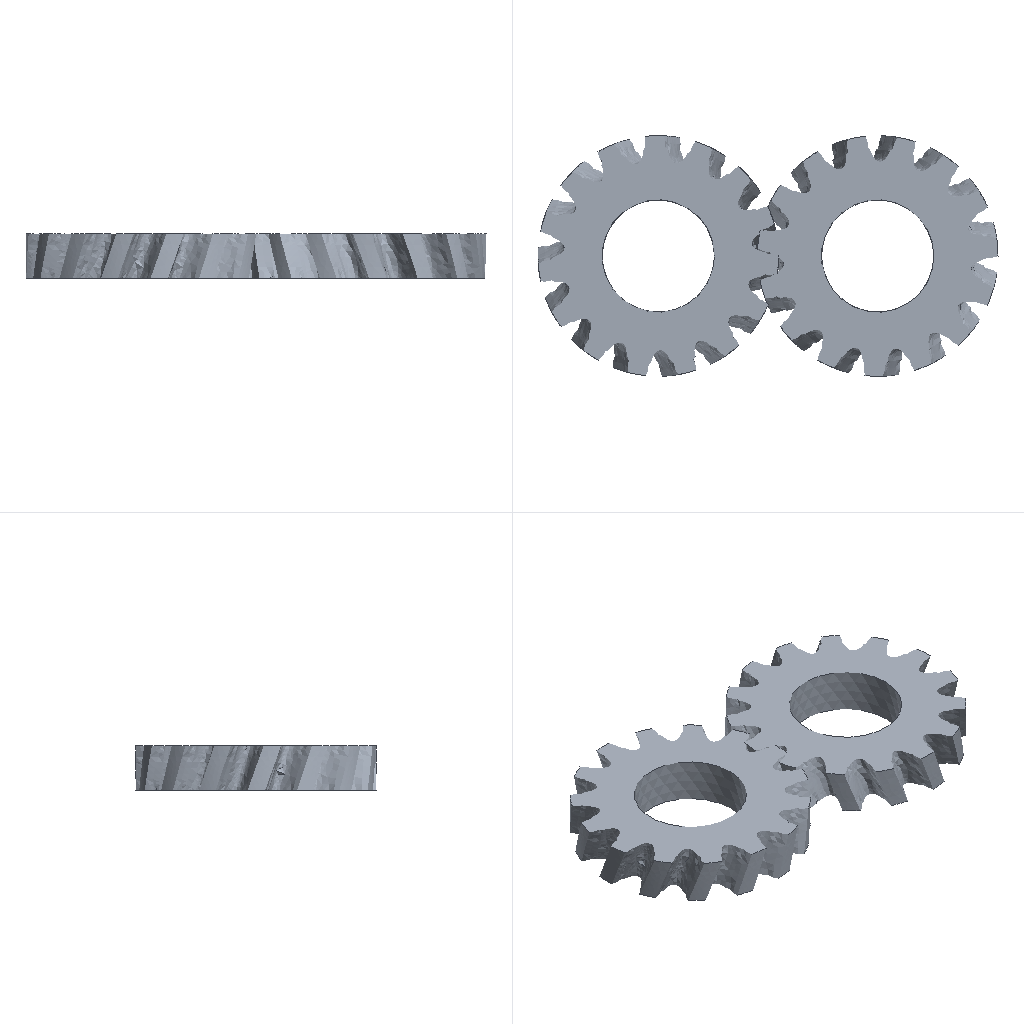Simulation study | ansys workbench
Ansys APDL input file, long lists of numbers shortened:
/batch
/config,noeldb,1     ! force off writing results to database
*get,_wallstrt,active,,time,wall
! ANSYS input file written by Workbench version 16.0 RELEASE
! File used for geometry attach: C:\Users\hmm\AppData\Local\Temp\WB_LAPTOP-92PEKBNI_hmm_19940_2\unsaved_project_files\dp0\SYS\DM\SYS.agdb
/title,unsaved_project--Static Structural (A5)
*DIM,_wb_ProjectScratch_dir,string,248
_wb_ProjectScratch_dir(1) = 'C:\Users\hmm\AppData\Local\Temp\WB_LAPTOP-92PEKBNI_hmm_19940_2\_ProjectScratch\Scr7DD3\'
*DIM,_wb_SolverFiles_dir,string,248
_wb_SolverFiles_dir(1) = 'C:\Users\hmm\AppData\Local\Temp\WB_LAPTOP-92PEKBNI_hmm_19940_2\unsaved_project_files\dp0\SYS\MECH\'
*DIM,_wb_userfiles_dir,string,248
_wb_userfiles_dir(1) = 'C:\Users\hmm\AppData\Local\Temp\WB_LAPTOP-92PEKBNI_hmm_19940_2\unsaved_project_files\user_files\'
/com,--- Data in consistent NMM units. See Solving Units in the help system for more information.
/units,MPA
/nopr
/wb,file,start              !  signify a WB generated input file
/prep7
! Turn off shape checking because checks already performed inside WB mesher.
! See help system for more information.
SHPP,OFF,,NOWARN
/nolist
etcon,set             ! allow ANSYS to choose best KEYOP's for 180x elements
/com,*********** Nodes for the whole assembly ***********
nblock,3
(1i9,3e20.9e3)
        1    6.183845739E+001   -1.519273240E+001    4.233906430E+000
! (51987 more lines like these left out)
-1
/wb,elem,start            !  set before creation of elements
/com,*********** Elements for Body 1 "Solid" ***********
et,1,187
eblock,19,solid,,11470
(19i9)
        1        1        1        1        0        0        0        0       10        0        1        2        8      444        9     4085     4078     4145     4116
! (22939 more lines like these left out)
-1
/com,*********** Elements for Body 2 "Solid" ***********
et,2,187
eblock,19,solid,,14800
(19i9)
        2        2        2        2        0        0        0        0       10        0    11471    23126    24680    25907    25826    28074    45158    28065    28080
! (29599 more lines like these left out)
-1
/wb,elem,end               !  done creating elements
/com,*********** Send User Defined Coordinate System(s) ***********
local,12,0,48.804,3.57140444047492e-015,5.,-0.,0.,0.
local,13,0,0.,-7.65404249467096e-016,5.,-0.,0.,0.
csys,0
toffst,273.15,  ! Temperature offset from absolute zero
/com,*********** Set Reference Temperature ***********
tref,22.
/wb,mat,start              !  starting to send materials
/com,*********** Send Materials ***********
MP,DENS,1,7.85e-09,	! tonne mm^-3
MP,ALPX,1,1.2e-05,	! C^-1
MP,C,1,434000000,	! mm^2 s^-2 C^-1
MP,KXX,1,60.5,	! tonne mm s^-3 C^-1
MP,RSVX,1,0.00017,	! ohm mm
MP,EX,1,200000,	! tonne s^-2 mm^-1
MP,NUXY,1,0.3,
MP,MURX,1,10000,
MP,DENS,2,7.85e-09,	! tonne mm^-3
MP,ALPX,2,1.2e-05,	! C^-1
MP,C,2,434000000,	! mm^2 s^-2 C^-1
MP,KXX,2,60.5,	! tonne mm s^-3 C^-1
MP,RSVX,2,0.00017,	! ohm mm
MP,EX,2,200000,	! tonne s^-2 mm^-1
MP,NUXY,2,0.3,
MP,MURX,2,10000,
/wb,mat,end                !  done sending materials
!************************* Model Summary ********************
!Solid,	Structural Steel,	matid,	1
!Solid,	Structural Steel,	matid,	2
!************************* End Model Summary ********************
! get the diagonal of the bounding box. Needed later for other things
*get,_xmin,node,,mnloc,x
*get,_ymin,node,,mnloc,y
*get,_zmin,node,,mnloc,z
*get,_xmax,node,,mxloc,x
*get,_ymax,node,,mxloc,y
*get,_zmax,node,,mxloc,z
_ASMDIAG=(_xmax-_xmin)*(_xmax-_xmin)+(_ymax-_ymin)*(_ymax-_ymin)+(_zmax-_zmin)*(_zmax-_zmin)
_ASMDIAG=SQRT(_ASMDIAG)
/wb,contact,start          !  starting to send contact
/com,*********** Create Contact "Frictional - No Selection To No Selection" ***********
/com,            Real Constant Set For Above Contact Is 4 & 3
*set,tid,4
*set,cid,3
r,tid
r,cid
et,tid,170
et,cid,174
eblock,10,,,3036
(15i9)
    26277        4        4        4        0     2495     2490     2493     2493    16197    16195     2493    16196
! (3035 more lines like these left out)
-1
eblock,10,,,3036
(15i9)
    29313        3        3        3        0     2495     2490     2493     2493    16197    16195     2493    16196
! (3035 more lines like these left out)
-1
eblock,10,,,4294
(15i9)
    32349        3        4        3        0    26571    26575    26578    26578    44256    44254    26578    44255
! (4293 more lines like these left out)
-1
eblock,10,,,4294
(15i9)
    36643        4        3        4        0    26571    26575    26578    26578    44256    44254    26578    44255
! (4293 more lines like these left out)
-1
keyo,cid,8,2               ! auto create asymmetric contact (from Program Controlled setting)
keyo,cid,10,2              ! adjust contact stiffness each NR iteration (from Program Controlled setting)
keyo,cid,12,0              ! standard contact
mp,mu,cid,0.1	! unitless
keyo,cid,2,0               ! augmented Lagrange (from Program Controlled setting)
keyo,cid,4,0               ! on Gauss point (from Program Controlled setting)
keyo,cid,9,0               ! use real geometry with stepped effects
keyo,cid,7,0               ! No Prediction
rmod,tid,3,1.	! FKN
rmod,tid,5,0.	! ICONT
rmod,tid,6,0.	! PINB
rmod,tid,10,0.	! CNOF
rmod,tid,12,0.	! FKT
rmod,tid,36,44	! WB DSID
rmod,cid,3,1.	! FKN
rmod,cid,5,0.	! ICONT
rmod,cid,6,0.	! PINB
rmod,cid,10,0.	! CNOF
rmod,cid,12,0.	! FKT
rmod,cid,36,44	! WB DSID
nsel,all
esel,all
/wb,contact,end            !  done creating contacts
/com,*********** Send Named Selection as Node Component ***********
CMBLOCK,SELECTION,NODE,     6867
(8i10)
        11        12       433       434       435       436       437       438
! (858 more lines like these left out)
/com,*********** Send Named Selection as Node Component ***********
CMBLOCK,SELECTION_2,NODE,     9383
(8i10)
     23134     23135     23141     23142     23143     23158     23169     23195
! (1172 more lines like these left out)
/golist
/wb,load,start             !  starting to send loads
nsel,all
/com,*********** Create Remote Point "Internal Remote Point 2" ***********
! -------- Remote Point Used by "Revolute - Ground To Solid" --------
*set,tid,6
*set,cid,5
et,cid,174
et,tid,170
keyo,tid,2,1               ! Don't fix the pilot node
keyo,tid,4,111111
keyo,cid,12,5              ! Bonded Contact
keyo,cid,4,2               ! Rigid CERIG style load
keyo,cid,2,2               ! MPC style contact
eblock,10,,,200
(15i9)
    40937        5        5        5        0     1337      704     1343     1343    22904    22894     1343    22901
! (199 more lines like these left out)
-1
*set,_npilot,51986
_npilot50=_npilot
type,tid
mat ,cid
real,cid
tshape,pilo
en,41137,_npilot
tshape
/com,*********** Create Remote Point "Internal Remote Point 4" ***********
! -------- Remote Point Used by "Revolute - Ground To Solid" --------
*set,tid,8
*set,cid,7
et,cid,174
et,tid,170
keyo,tid,2,1               ! Don't fix the pilot node
keyo,tid,4,111111
keyo,cid,12,5              ! Bonded Contact
keyo,cid,4,2               ! Rigid CERIG style load
keyo,cid,2,2               ! MPC style contact
eblock,10,,,200
(15i9)
    41138        7        7        7        0    24651    25201    25240    25240    51943    51513    25240    51942
! (199 more lines like these left out)
-1
*set,_npilot,51988
_npilot57=_npilot
type,tid
mat ,cid
real,cid
tshape,pilo
en,41338,_npilot
tshape
/com,*********** Create Joint "Revolute - Ground To Solid" ***********
/com,            Real Constant Set For Above Joint Is 9
! Joint Element Type Declaration and Definition using MPC184
*set,_jid,9
et,_jid,184
keyo,_jid,1,6           ! Revolute Joint
keyo,_jid,4,1           ! Z Axis is revolute axis
sectype,_jid, joint, revo, _wbjoint
secjoint,,12,12
mat,_jid
real,_jid
type,_jid
secnum,_jid
en,26273,,51986        ! body to ground joint
/com,*********** Create Joint "Revolute - Ground To Solid" ***********
/com,            Real Constant Set For Above Joint Is 10
! Joint Element Type Declaration and Definition using MPC184
*set,_jid,10
et,_jid,184
keyo,_jid,1,6           ! Revolute Joint
keyo,_jid,4,1           ! Z Axis is revolute axis
sectype,_jid, joint, revo, _wbjoint
secjoint,,13,13
mat,_jid
real,_jid
type,_jid
secnum,_jid
en,26276,,51988        ! body to ground joint
et,11,14             ! spring element type
/com,*********** Construct Weak Springs, Prototype 1 ***********
*set,_delta,3.815
type,11
mat,12
real,12
r,12,2.1153666700045e-004
nsel,all
*get,_nspr,ndmx
_nspr=_nspr+1
esel,s,mat,,1
nsle,s,active
*get,_minx,node,0,mnloc,x
*get,_miny,node,0,mnloc,y
*get,_minz,node,0,mnloc,z
*get,_maxx,node,0,mxloc,x
*get,_maxy,node,0,mxloc,y
*get,_maxz,node,0,mxloc,z
*dim,_ntets,arra,8
_ntets(1) = NODE(_minx,_miny,_minz)
_ntets(2) = NODE(_minx,_miny,_maxz)
_ntets(3) = NODE(_minx,_maxy,_minz)
_ntets(4) = NODE(_minx,_maxy,_maxz)
_ntets(5) = NODE(_maxx,_miny,_minz)
_ntets(6) = NODE(_maxx,_miny,_maxz)
_ntets(7) = NODE(_maxx,_maxy,_minz)
_ntets(8) = NODE(_maxx,_maxy,_maxz)
*do,_i,1,8
  n,_nspr,nx(_ntets(_i))+_delta,ny(_ntets(_i)),nz(_ntets(_i))
  e,_ntets(_i),_nspr
  d,_nspr,all
  _nspr=_nspr+1
  n,_nspr,nx(_ntets(_i)),ny(_ntets(_i))+_delta,nz(_ntets(_i))
  e,_ntets(_i),_nspr
  d,_nspr,all
  _nspr=_nspr+1
  n,_nspr,nx(_ntets(_i)),ny(_ntets(_i)),nz(_ntets(_i))+_delta
  e,_ntets(_i),_nspr
  d,_nspr,all
  _nspr=_nspr+1
*enddo
*set,_ntets
nsel,all
esel,all
/com,*********** Construct Weak Springs, Prototype 2 ***********
*set,_delta,3.815
type,11
mat,13
real,13
r,13,1.94305589646612e-004
nsel,all
*get,_nspr,ndmx
_nspr=_nspr+1
esel,s,mat,,2
nsle,s,active
*get,_minx,node,0,mnloc,x
*get,_miny,node,0,mnloc,y
*get,_minz,node,0,mnloc,z
*get,_maxx,node,0,mxloc,x
*get,_maxy,node,0,mxloc,y
*get,_maxz,node,0,mxloc,z
*dim,_ntets,arra,8
_ntets(1) = NODE(_minx,_miny,_minz)
_ntets(2) = NODE(_minx,_miny,_maxz)
_ntets(3) = NODE(_minx,_maxy,_minz)
_ntets(4) = NODE(_minx,_maxy,_maxz)
_ntets(5) = NODE(_maxx,_miny,_minz)
_ntets(6) = NODE(_maxx,_miny,_maxz)
_ntets(7) = NODE(_maxx,_maxy,_minz)
_ntets(8) = NODE(_maxx,_maxy,_maxz)
*do,_i,1,8
  n,_nspr,nx(_ntets(_i))+_delta,ny(_ntets(_i)),nz(_ntets(_i))
  e,_ntets(_i),_nspr
  d,_nspr,all
  _nspr=_nspr+1
  n,_nspr,nx(_ntets(_i)),ny(_ntets(_i))+_delta,nz(_ntets(_i))
  e,_ntets(_i),_nspr
  d,_nspr,all
  _nspr=_nspr+1
  n,_nspr,nx(_ntets(_i)),ny(_ntets(_i)),nz(_ntets(_i))+_delta
  e,_ntets(_i),_nspr
  d,_nspr,all
  _nspr=_nspr+1
*enddo
*set,_ntets
nsel,all
esel,all
/com,*********** Create Joint Drivers **********
*DIM,_loadvari62,TABLE,2,1,1,TIME,
! Time values
_loadvari62(1,0,1) = 0.
_loadvari62(2,0,1) = 1.
! Load values
_loadvari62(1,1,1) = 0.
_loadvari62(2,1,1) = 0.
*DIM,_loadvari63,TABLE,2,1,1,TIME,
! Time values
_loadvari63(1,0,1) = 0.
_loadvari63(2,0,1) = 1.
! Load values
_loadvari63(1,1,1) = 0.
_loadvari63(2,1,1) = 0.
/gst,on,on
fini
*get,_numnode,node,0,count
*get,_numelem,elem,0,count
*get, _MAXELEMNUM, elem, 0, NUM, MAX
*get, _MAXNODENUM, node, 0, NUM, MAX
*get, _MAXELEMTYPE, etyp, 0, NUM, MAX
*get, _MAXREALCONST, real, 0, NUM, MAX
/go
/wb,load,end               !  done creating loads
/com,--- Number of total nodes = %_numnode%
/com,--- Number of contact elements = 15060
/com,--- Number of spring elements = 48
/com,--- Number of bearing elements = 0
/com,--- Number of solid elements = 26270
/com,--- Number of total elements = %_numelem%
*get,_wallbsol,active,,time,wall
/com,****************************************************************************
/com,*************************    SOLUTION       ********************************
/com,****************************************************************************
/solu
antype,0                   ! static analysis
eqsl,pcg,1e-8,,,,,,1
cntr,print,1               ! print out contact info and also make no initial contact an error
nldiag,cont,iter           ! print out contact info each equilibrium iteration
resc,define,last,last,,dele	   ! Program Controlled
/com,****************************************************
/com,******************* SOLVE FOR LS 1 ****************
/nopr
/gopr
esel,s,type,,9
dj,all,rotz,%_loadvari62%
esel,all
esel,s,type,,10
dj,all,rotz,%_loadvari63%
esel,all
autots,on                   ! User turned on automatic time stepping
nsub,5,5,5,OFF
time,1.
outres,erase
outres,all,none
outres,nsol,all
outres,rsol,all
outres,strs,all
outres,epel,all
outres,eppl,all
/nopr
esel,s,mat,,9
esel,a,mat,,10
cm,_elmisc,elem
esel,all
/gopr
outres,misc,all,_elmisc
stabilize,off                   ! Stabilization turned OFF by user
! *********** WB SOLVE COMMAND ***********
! check interactive state
*get,ANSINTER_,active,,int
*if,ANSINTER_,ne,0,then
/eof
*endif
solve
/com *************** Write FE CONNECTORS *********
CEWRITE,file,ce,,INTE
/com,****************************************************
/com,*************** FINISHED SOLVE FOR LS 1 *************
*set,_DS_PROGRESS          ! turn off progress updates to avoid virus scanning bug
*get,_wallasol,active,,time,wall
/nopr
*get,_numnode,node,0,count
*get,_numelem,elem,0,count
*get, _MAXELEMNUM, elem, 0, NUM, MAX
*get, _MAXNODENUM, node, 0, NUM, MAX,,,INTERNAL
*get, _MAXELEMTYPE, etyp, 0, NUM, MAX
*get, _MAXREALCONST, real, 0, NUM, MAX
/gopr
*get,_PCGITER,active,,solu,cgiter
/post1
xmlo,ENCODING,ISO-8859-1
xmlo,parm
/xml,parm,xml
fini
/gopr
*get,_walldone,active,,time,wall
_preptime=(_wallbsol-_wallstrt)*3600
_solvtime=(_wallasol-_wallbsol)*3600
_posttime=(_walldone-_wallasol)*3600
_totaltim=(_walldone-_wallstrt)*3600
/wb,file,end               ! done with WB generated input